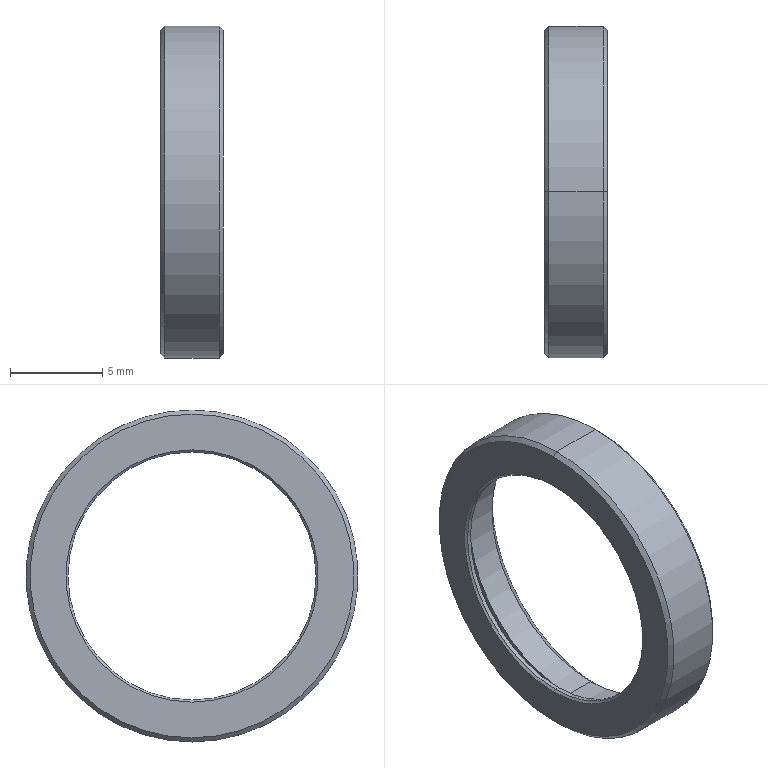Part | SolidWorks | features Revolution 1 | 1 solid | 20 faces | box 3.414 x 18 x 18 mm | volume 239.463 mm3 | cylinder 8 | cone 8 | plane 4 | commonest cylinder face diameters 13.448 x2 15.155 x2 15.951 x2 18 x2
STEP:
#1=CARTESIAN_POINT('',(1545.039,1902.873,9.));
#2=VERTEX_POINT('',#1);
#3=CARTESIAN_POINT('',(1545.039,1902.873,-9.));
#4=VERTEX_POINT('',#3);
#5=CARTESIAN_POINT('',(1545.039,1902.873,0.));
#6=DIRECTION('',(-1.,0.,0.));
#7=DIRECTION('',(0.,0.,1.));
#8=AXIS2_PLACEMENT_3D('',#5,#6,#7);
#9=CIRCLE('',#8,9.);
#10=EDGE_CURVE('',#2,#4,#9,.T.);
#11=ORIENTED_EDGE('',*,*,#10,.T.);
#12=CARTESIAN_POINT('',(1542.08,1902.873,-9.));
#13=VERTEX_POINT('',#12);
#14=CARTESIAN_POINT('',(1539.353,1902.873,-9.));
#15=DIRECTION('',(-1.,0.,0.));
#16=VECTOR('',#15,1000.);
#17=LINE('',#14,#16);
#18=EDGE_CURVE('',#4,#13,#17,.T.);
#19=ORIENTED_EDGE('',*,*,#18,.T.);
#20=CARTESIAN_POINT('',(1542.08,1902.873,9.));
#21=VERTEX_POINT('',#20);
#22=CARTESIAN_POINT('',(1542.08,1902.873,0.));
#23=DIRECTION('',(-1.,0.,0.));
#24=DIRECTION('',(0.,0.,1.));
#25=AXIS2_PLACEMENT_3D('',#22,#23,#24);
#26=CIRCLE('',#25,9.);
#27=EDGE_CURVE('',#21,#13,#26,.T.);
#28=ORIENTED_EDGE('',*,*,#27,.F.);
#29=CARTESIAN_POINT('',(1539.353,1902.873,9.));
#30=DIRECTION('',(-1.,0.,0.));
#31=VECTOR('',#30,1000.);
#32=LINE('',#29,#31);
#33=EDGE_CURVE('',#2,#21,#32,.T.);
#34=ORIENTED_EDGE('',*,*,#33,.F.);
#35=EDGE_LOOP('',(#11,#19,#28,#34));
#36=FACE_OUTER_BOUND('',#35,.T.);
#37=CARTESIAN_POINT('',(1539.353,1902.873,0.));
#38=DIRECTION('',(-1.,0.,0.));
#39=DIRECTION('',(0.,0.,1.));
#40=AXIS2_PLACEMENT_3D('',#37,#38,#39);
#41=CYLINDRICAL_SURFACE('',#40,9.);
#42=ADVANCED_FACE('',(#36),#41,.T.);
#43=CARTESIAN_POINT('',(1541.852,1902.873,8.772));
#44=VERTEX_POINT('',#43);
#45=CARTESIAN_POINT('',(1541.852,1902.873,-8.772));
#46=VERTEX_POINT('',#45);
#47=CARTESIAN_POINT('',(1541.852,1902.873,0.));
#48=DIRECTION('',(-1.,0.,0.));
#49=DIRECTION('',(0.,0.,1.));
#50=AXIS2_PLACEMENT_3D('',#47,#48,#49);
#51=CIRCLE('',#50,8.772);
#52=EDGE_CURVE('',#44,#46,#51,.T.);
#53=ORIENTED_EDGE('',*,*,#52,.F.);
#54=CARTESIAN_POINT('',(1541.852,1902.873,8.772));
#55=DIRECTION('',(0.7071,0.,0.7071));
#56=VECTOR('',#55,1000.);
#57=LINE('',#54,#56);
#58=EDGE_CURVE('',#44,#21,#57,.T.);
#59=ORIENTED_EDGE('',*,*,#58,.T.);
#60=ORIENTED_EDGE('',*,*,#27,.T.);
#61=CARTESIAN_POINT('',(1541.852,1902.873,-8.772));
#62=DIRECTION('',(0.7071,0.,-0.7071));
#63=VECTOR('',#62,1000.);
#64=LINE('',#61,#63);
#65=EDGE_CURVE('',#46,#13,#64,.T.);
#66=ORIENTED_EDGE('',*,*,#65,.F.);
#67=EDGE_LOOP('',(#53,#59,#60,#66));
#68=FACE_OUTER_BOUND('',#67,.T.);
#69=CARTESIAN_POINT('',(1541.852,1902.873,0.));
#70=DIRECTION('',(1.,0.,0.));
#71=DIRECTION('',(0.,0.,-1.));
#72=AXIS2_PLACEMENT_3D('',#69,#70,#71);
#73=CONICAL_SURFACE('',#72,8.772,0.7854);
#74=ADVANCED_FACE('',(#68),#73,.T.);
#75=CARTESIAN_POINT('',(1541.966,1902.873,-6.724));
#76=VERTEX_POINT('',#75);
#77=CARTESIAN_POINT('',(1541.966,1902.873,6.724));
#78=VERTEX_POINT('',#77);
#79=CARTESIAN_POINT('',(1541.966,1902.873,0.));
#80=DIRECTION('',(-1.,0.,0.));
#81=DIRECTION('',(0.,0.,1.));
#82=AXIS2_PLACEMENT_3D('',#79,#80,#81);
#83=CIRCLE('',#82,6.724);
#84=EDGE_CURVE('',#76,#78,#83,.T.);
#85=ORIENTED_EDGE('',*,*,#84,.F.);
#86=CARTESIAN_POINT('',(1541.852,1902.873,-6.838));
#87=VERTEX_POINT('',#86);
#88=CARTESIAN_POINT('',(1541.966,1902.873,-6.724));
#89=DIRECTION('',(-0.7071,0.,-0.7071));
#90=VECTOR('',#89,1000.);
#91=LINE('',#88,#90);
#92=EDGE_CURVE('',#76,#87,#91,.T.);
#93=ORIENTED_EDGE('',*,*,#92,.T.);
#94=CARTESIAN_POINT('',(1541.852,1902.873,6.838));
#95=VERTEX_POINT('',#94);
#96=CARTESIAN_POINT('',(1541.852,1902.873,0.));
#97=DIRECTION('',(-1.,0.,0.));
#98=DIRECTION('',(0.,0.,1.));
#99=AXIS2_PLACEMENT_3D('',#96,#97,#98);
#100=CIRCLE('',#99,6.838);
#101=EDGE_CURVE('',#87,#95,#100,.T.);
#102=ORIENTED_EDGE('',*,*,#101,.T.);
#103=CARTESIAN_POINT('',(1541.966,1902.873,6.724));
#104=DIRECTION('',(-0.7071,0.,0.7071));
#105=VECTOR('',#104,1000.);
#106=LINE('',#103,#105);
#107=EDGE_CURVE('',#78,#95,#106,.T.);
#108=ORIENTED_EDGE('',*,*,#107,.F.);
#109=EDGE_LOOP('',(#85,#93,#102,#108));
#110=FACE_OUTER_BOUND('',#109,.T.);
#111=CARTESIAN_POINT('',(1541.966,1902.873,0.));
#112=DIRECTION('',(-1.,0.,0.));
#113=DIRECTION('',(0.,0.,1.));
#114=AXIS2_PLACEMENT_3D('',#111,#112,#113);
#115=CONICAL_SURFACE('',#114,6.724,0.7854);
#116=ADVANCED_FACE('',(#110),#115,.F.);
#117=CARTESIAN_POINT('',(1542.194,1902.873,-6.724));
#118=VERTEX_POINT('',#117);
#119=CARTESIAN_POINT('',(1542.194,1902.873,6.724));
#120=VERTEX_POINT('',#119);
#121=CARTESIAN_POINT('',(1542.194,1902.873,0.));
#122=DIRECTION('',(-1.,0.,0.));
#123=DIRECTION('',(0.,0.,1.));
#124=AXIS2_PLACEMENT_3D('',#121,#122,#123);
#125=CIRCLE('',#124,6.724);
#126=EDGE_CURVE('',#118,#120,#125,.T.);
#127=ORIENTED_EDGE('',*,*,#126,.F.);
#128=CARTESIAN_POINT('',(1539.353,1902.873,-6.724));
#129=DIRECTION('',(-1.,0.,0.));
#130=VECTOR('',#129,1000.);
#131=LINE('',#128,#130);
#132=EDGE_CURVE('',#118,#76,#131,.T.);
#133=ORIENTED_EDGE('',*,*,#132,.T.);
#134=ORIENTED_EDGE('',*,*,#84,.T.);
#135=CARTESIAN_POINT('',(1539.353,1902.873,6.724));
#136=DIRECTION('',(-1.,0.,0.));
#137=VECTOR('',#136,1000.);
#138=LINE('',#135,#137);
#139=EDGE_CURVE('',#120,#78,#138,.T.);
#140=ORIENTED_EDGE('',*,*,#139,.F.);
#141=EDGE_LOOP('',(#127,#133,#134,#140));
#142=FACE_OUTER_BOUND('',#141,.T.);
#143=CARTESIAN_POINT('',(1539.353,1902.873,0.));
#144=DIRECTION('',(-1.,0.,0.));
#145=DIRECTION('',(0.,0.,1.));
#146=AXIS2_PLACEMENT_3D('',#143,#144,#145);
#147=CYLINDRICAL_SURFACE('',#146,6.724);
#148=ADVANCED_FACE('',(#142),#147,.F.);
#149=CARTESIAN_POINT('',(1542.99,1902.873,-7.976));
#150=VERTEX_POINT('',#149);
#151=CARTESIAN_POINT('',(1542.99,1902.873,7.976));
#152=VERTEX_POINT('',#151);
#153=CARTESIAN_POINT('',(1542.99,1902.873,0.));
#154=DIRECTION('',(-1.,0.,0.));
#155=DIRECTION('',(0.,0.,1.));
#156=AXIS2_PLACEMENT_3D('',#153,#154,#155);
#157=CIRCLE('',#156,7.976);
#158=EDGE_CURVE('',#150,#152,#157,.T.);
#159=ORIENTED_EDGE('',*,*,#158,.F.);
#160=CARTESIAN_POINT('',(1542.194,1902.873,-7.976));
#161=VERTEX_POINT('',#160);
#162=CARTESIAN_POINT('',(1539.353,1902.873,-7.976));
#163=DIRECTION('',(-1.,0.,0.));
#164=VECTOR('',#163,1000.);
#165=LINE('',#162,#164);
#166=EDGE_CURVE('',#150,#161,#165,.T.);
#167=ORIENTED_EDGE('',*,*,#166,.T.);
#168=CARTESIAN_POINT('',(1542.194,1902.873,7.976));
#169=VERTEX_POINT('',#168);
#170=CARTESIAN_POINT('',(1542.194,1902.873,0.));
#171=DIRECTION('',(-1.,0.,0.));
#172=DIRECTION('',(0.,0.,1.));
#173=AXIS2_PLACEMENT_3D('',#170,#171,#172);
#174=CIRCLE('',#173,7.976);
#175=EDGE_CURVE('',#161,#169,#174,.T.);
#176=ORIENTED_EDGE('',*,*,#175,.T.);
#177=CARTESIAN_POINT('',(1539.353,1902.873,7.976));
#178=DIRECTION('',(-1.,0.,0.));
#179=VECTOR('',#178,1000.);
#180=LINE('',#177,#179);
#181=EDGE_CURVE('',#152,#169,#180,.T.);
#182=ORIENTED_EDGE('',*,*,#181,.F.);
#183=EDGE_LOOP('',(#159,#167,#176,#182));
#184=FACE_OUTER_BOUND('',#183,.T.);
#185=CARTESIAN_POINT('',(1539.353,1902.873,0.));
#186=DIRECTION('',(-1.,0.,0.));
#187=DIRECTION('',(0.,0.,1.));
#188=AXIS2_PLACEMENT_3D('',#185,#186,#187);
#189=CYLINDRICAL_SURFACE('',#188,7.976);
#190=ADVANCED_FACE('',(#184),#189,.F.);
#191=CARTESIAN_POINT('',(1544.697,1902.873,-7.577));
#192=VERTEX_POINT('',#191);
#193=CARTESIAN_POINT('',(1544.697,1902.873,7.577));
#194=VERTEX_POINT('',#193);
#195=CARTESIAN_POINT('',(1544.697,1902.873,0.));
#196=DIRECTION('',(-1.,0.,0.));
#197=DIRECTION('',(0.,0.,1.));
#198=AXIS2_PLACEMENT_3D('',#195,#196,#197);
#199=CIRCLE('',#198,7.577);
#200=EDGE_CURVE('',#192,#194,#199,.T.);
#201=ORIENTED_EDGE('',*,*,#200,.F.);
#202=CARTESIAN_POINT('',(1542.99,1902.873,-7.577));
#203=VERTEX_POINT('',#202);
#204=CARTESIAN_POINT('',(1539.353,1902.873,-7.577));
#205=DIRECTION('',(-1.,0.,0.));
#206=VECTOR('',#205,1000.);
#207=LINE('',#204,#206);
#208=EDGE_CURVE('',#192,#203,#207,.T.);
#209=ORIENTED_EDGE('',*,*,#208,.T.);
#210=CARTESIAN_POINT('',(1542.99,1902.873,7.577));
#211=VERTEX_POINT('',#210);
#212=CARTESIAN_POINT('',(1542.99,1902.873,0.));
#213=DIRECTION('',(-1.,0.,0.));
#214=DIRECTION('',(0.,0.,1.));
#215=AXIS2_PLACEMENT_3D('',#212,#213,#214);
#216=CIRCLE('',#215,7.577);
#217=EDGE_CURVE('',#203,#211,#216,.T.);
#218=ORIENTED_EDGE('',*,*,#217,.T.);
#219=CARTESIAN_POINT('',(1539.353,1902.873,7.577));
#220=DIRECTION('',(-1.,0.,0.));
#221=VECTOR('',#220,1000.);
#222=LINE('',#219,#221);
#223=EDGE_CURVE('',#194,#211,#222,.T.);
#224=ORIENTED_EDGE('',*,*,#223,.F.);
#225=EDGE_LOOP('',(#201,#209,#218,#224));
#226=FACE_OUTER_BOUND('',#225,.T.);
#227=CARTESIAN_POINT('',(1539.353,1902.873,0.));
#228=DIRECTION('',(-1.,0.,0.));
#229=DIRECTION('',(0.,0.,1.));
#230=AXIS2_PLACEMENT_3D('',#227,#228,#229);
#231=CYLINDRICAL_SURFACE('',#230,7.577);
#232=ADVANCED_FACE('',(#226),#231,.F.);
#233=ORIENTED_EDGE('',*,*,#200,.T.);
#234=CARTESIAN_POINT('',(1545.266,1902.873,8.146));
#235=VERTEX_POINT('',#234);
#236=CARTESIAN_POINT('',(1545.266,1902.873,8.146));
#237=DIRECTION('',(0.7071,0.,0.7071));
#238=VECTOR('',#237,1000.);
#239=LINE('',#236,#238);
#240=EDGE_CURVE('',#194,#235,#239,.T.);
#241=ORIENTED_EDGE('',*,*,#240,.T.);
#242=CARTESIAN_POINT('',(1545.266,1902.873,-8.146));
#243=VERTEX_POINT('',#242);
#244=CARTESIAN_POINT('',(1545.266,1902.873,0.));
#245=DIRECTION('',(-1.,0.,0.));
#246=DIRECTION('',(0.,0.,1.));
#247=AXIS2_PLACEMENT_3D('',#244,#245,#246);
#248=CIRCLE('',#247,8.146);
#249=EDGE_CURVE('',#243,#235,#248,.T.);
#250=ORIENTED_EDGE('',*,*,#249,.F.);
#251=CARTESIAN_POINT('',(1545.266,1902.873,-8.146));
#252=DIRECTION('',(0.7071,0.,-0.7071));
#253=VECTOR('',#252,1000.);
#254=LINE('',#251,#253);
#255=EDGE_CURVE('',#192,#243,#254,.T.);
#256=ORIENTED_EDGE('',*,*,#255,.F.);
#257=EDGE_LOOP('',(#233,#241,#250,#256));
#258=FACE_OUTER_BOUND('',#257,.T.);
#259=CARTESIAN_POINT('',(1545.266,1902.873,0.));
#260=DIRECTION('',(1.,0.,0.));
#261=DIRECTION('',(0.,0.,-1.));
#262=AXIS2_PLACEMENT_3D('',#259,#260,#261);
#263=CONICAL_SURFACE('',#262,8.146,0.7854);
#264=ADVANCED_FACE('',(#258),#263,.F.);
#265=CARTESIAN_POINT('',(1545.266,1902.873,8.772));
#266=VERTEX_POINT('',#265);
#267=CARTESIAN_POINT('',(1545.266,1902.873,-8.772));
#268=VERTEX_POINT('',#267);
#269=CARTESIAN_POINT('',(1545.266,1902.873,0.));
#270=DIRECTION('',(-1.,0.,0.));
#271=DIRECTION('',(0.,0.,1.));
#272=AXIS2_PLACEMENT_3D('',#269,#270,#271);
#273=CIRCLE('',#272,8.772);
#274=EDGE_CURVE('',#266,#268,#273,.T.);
#275=ORIENTED_EDGE('',*,*,#274,.T.);
#276=CARTESIAN_POINT('',(1545.266,1902.873,-8.772));
#277=DIRECTION('',(-0.7071,0.,-0.7071));
#278=VECTOR('',#277,1000.);
#279=LINE('',#276,#278);
#280=EDGE_CURVE('',#268,#4,#279,.T.);
#281=ORIENTED_EDGE('',*,*,#280,.T.);
#282=ORIENTED_EDGE('',*,*,#10,.F.);
#283=CARTESIAN_POINT('',(1545.266,1902.873,8.772));
#284=DIRECTION('',(-0.7071,0.,0.7071));
#285=VECTOR('',#284,1000.);
#286=LINE('',#283,#285);
#287=EDGE_CURVE('',#266,#2,#286,.T.);
#288=ORIENTED_EDGE('',*,*,#287,.F.);
#289=EDGE_LOOP('',(#275,#281,#282,#288));
#290=FACE_OUTER_BOUND('',#289,.T.);
#291=CARTESIAN_POINT('',(1545.266,1902.873,0.));
#292=DIRECTION('',(-1.,0.,0.));
#293=DIRECTION('',(0.,0.,1.));
#294=AXIS2_PLACEMENT_3D('',#291,#292,#293);
#295=CONICAL_SURFACE('',#294,8.772,0.7854);
#296=ADVANCED_FACE('',(#290),#295,.T.);
#297=ORIENTED_EDGE('',*,*,#280,.F.);
#298=CARTESIAN_POINT('',(1545.266,1902.873,0.));
#299=DIRECTION('',(-1.,0.,0.));
#300=DIRECTION('',(0.,0.,1.));
#301=AXIS2_PLACEMENT_3D('',#298,#299,#300);
#302=CIRCLE('',#301,8.772);
#303=EDGE_CURVE('',#268,#266,#302,.T.);
#304=ORIENTED_EDGE('',*,*,#303,.T.);
#305=ORIENTED_EDGE('',*,*,#287,.T.);
#306=CARTESIAN_POINT('',(1545.039,1902.873,0.));
#307=DIRECTION('',(-1.,0.,0.));
#308=DIRECTION('',(0.,0.,1.));
#309=AXIS2_PLACEMENT_3D('',#306,#307,#308);
#310=CIRCLE('',#309,9.);
#311=EDGE_CURVE('',#4,#2,#310,.T.);
#312=ORIENTED_EDGE('',*,*,#311,.F.);
#313=EDGE_LOOP('',(#297,#304,#305,#312));
#314=FACE_OUTER_BOUND('',#313,.T.);
#315=CARTESIAN_POINT('',(1545.266,1902.873,0.));
#316=DIRECTION('',(-1.,0.,0.));
#317=DIRECTION('',(0.,0.,1.));
#318=AXIS2_PLACEMENT_3D('',#315,#316,#317);
#319=CONICAL_SURFACE('',#318,8.772,0.7854);
#320=ADVANCED_FACE('',(#314),#319,.T.);
#321=ORIENTED_EDGE('',*,*,#274,.F.);
#322=ORIENTED_EDGE('',*,*,#303,.F.);
#323=EDGE_LOOP('',(#321,#322));
#324=FACE_OUTER_BOUND('',#323,.T.);
#325=ORIENTED_EDGE('',*,*,#249,.T.);
#326=CARTESIAN_POINT('',(1545.266,1902.873,0.));
#327=DIRECTION('',(-1.,0.,0.));
#328=DIRECTION('',(0.,0.,1.));
#329=AXIS2_PLACEMENT_3D('',#326,#327,#328);
#330=CIRCLE('',#329,8.146);
#331=EDGE_CURVE('',#235,#243,#330,.T.);
#332=ORIENTED_EDGE('',*,*,#331,.T.);
#333=EDGE_LOOP('',(#325,#332));
#334=FACE_BOUND('',#333,.T.);
#335=CARTESIAN_POINT('',(1545.266,-0.000000002,0.));
#336=DIRECTION('',(-1.,0.,0.));
#337=DIRECTION('',(0.,0.,1.));
#338=AXIS2_PLACEMENT_3D('',#335,#336,#337);
#339=PLANE('',#338);
#340=ADVANCED_FACE('',(#324,#334),#339,.F.);
#341=ORIENTED_EDGE('',*,*,#240,.F.);
#342=CARTESIAN_POINT('',(1544.697,1902.873,0.));
#343=DIRECTION('',(-1.,0.,0.));
#344=DIRECTION('',(0.,0.,1.));
#345=AXIS2_PLACEMENT_3D('',#342,#343,#344);
#346=CIRCLE('',#345,7.577);
#347=EDGE_CURVE('',#194,#192,#346,.T.);
#348=ORIENTED_EDGE('',*,*,#347,.T.);
#349=ORIENTED_EDGE('',*,*,#255,.T.);
#350=ORIENTED_EDGE('',*,*,#331,.F.);
#351=EDGE_LOOP('',(#341,#348,#349,#350));
#352=FACE_OUTER_BOUND('',#351,.T.);
#353=CARTESIAN_POINT('',(1545.266,1902.873,0.));
#354=DIRECTION('',(1.,0.,0.));
#355=DIRECTION('',(0.,0.,-1.));
#356=AXIS2_PLACEMENT_3D('',#353,#354,#355);
#357=CONICAL_SURFACE('',#356,8.146,0.7854);
#358=ADVANCED_FACE('',(#352),#357,.F.);
#359=ORIENTED_EDGE('',*,*,#208,.F.);
#360=ORIENTED_EDGE('',*,*,#347,.F.);
#361=ORIENTED_EDGE('',*,*,#223,.T.);
#362=CARTESIAN_POINT('',(1542.99,1902.873,0.));
#363=DIRECTION('',(-1.,0.,0.));
#364=DIRECTION('',(0.,0.,1.));
#365=AXIS2_PLACEMENT_3D('',#362,#363,#364);
#366=CIRCLE('',#365,7.577);
#367=EDGE_CURVE('',#211,#203,#366,.T.);
#368=ORIENTED_EDGE('',*,*,#367,.T.);
#369=EDGE_LOOP('',(#359,#360,#361,#368));
#370=FACE_OUTER_BOUND('',#369,.T.);
#371=CARTESIAN_POINT('',(1539.353,1902.873,0.));
#372=DIRECTION('',(-1.,0.,0.));
#373=DIRECTION('',(0.,0.,1.));
#374=AXIS2_PLACEMENT_3D('',#371,#372,#373);
#375=CYLINDRICAL_SURFACE('',#374,7.577);
#376=ADVANCED_FACE('',(#370),#375,.F.);
#377=CARTESIAN_POINT('',(1542.99,1902.873,0.));
#378=DIRECTION('',(-1.,0.,0.));
#379=DIRECTION('',(0.,0.,1.));
#380=AXIS2_PLACEMENT_3D('',#377,#378,#379);
#381=CIRCLE('',#380,7.976);
#382=EDGE_CURVE('',#152,#150,#381,.T.);
#383=ORIENTED_EDGE('',*,*,#382,.T.);
#384=ORIENTED_EDGE('',*,*,#158,.T.);
#385=EDGE_LOOP('',(#383,#384));
#386=FACE_OUTER_BOUND('',#385,.T.);
#387=ORIENTED_EDGE('',*,*,#367,.F.);
#388=ORIENTED_EDGE('',*,*,#217,.F.);
#389=EDGE_LOOP('',(#387,#388));
#390=FACE_BOUND('',#389,.T.);
#391=CARTESIAN_POINT('',(1542.99,0.,0.));
#392=DIRECTION('',(-1.,0.,0.));
#393=DIRECTION('',(0.,0.,1.));
#394=AXIS2_PLACEMENT_3D('',#391,#392,#393);
#395=PLANE('',#394);
#396=ADVANCED_FACE('',(#386,#390),#395,.T.);
#397=ORIENTED_EDGE('',*,*,#166,.F.);
#398=ORIENTED_EDGE('',*,*,#382,.F.);
#399=ORIENTED_EDGE('',*,*,#181,.T.);
#400=CARTESIAN_POINT('',(1542.194,1902.873,0.));
#401=DIRECTION('',(-1.,0.,0.));
#402=DIRECTION('',(0.,0.,1.));
#403=AXIS2_PLACEMENT_3D('',#400,#401,#402);
#404=CIRCLE('',#403,7.976);
#405=EDGE_CURVE('',#169,#161,#404,.T.);
#406=ORIENTED_EDGE('',*,*,#405,.T.);
#407=EDGE_LOOP('',(#397,#398,#399,#406));
#408=FACE_OUTER_BOUND('',#407,.T.);
#409=CARTESIAN_POINT('',(1539.353,1902.873,0.));
#410=DIRECTION('',(-1.,0.,0.));
#411=DIRECTION('',(0.,0.,1.));
#412=AXIS2_PLACEMENT_3D('',#409,#410,#411);
#413=CYLINDRICAL_SURFACE('',#412,7.976);
#414=ADVANCED_FACE('',(#408),#413,.F.);
#415=ORIENTED_EDGE('',*,*,#405,.F.);
#416=ORIENTED_EDGE('',*,*,#175,.F.);
#417=EDGE_LOOP('',(#415,#416));
#418=FACE_OUTER_BOUND('',#417,.T.);
#419=CARTESIAN_POINT('',(1542.194,1902.873,0.));
#420=DIRECTION('',(-1.,0.,0.));
#421=DIRECTION('',(0.,0.,1.));
#422=AXIS2_PLACEMENT_3D('',#419,#420,#421);
#423=CIRCLE('',#422,6.724);
#424=EDGE_CURVE('',#120,#118,#423,.T.);
#425=ORIENTED_EDGE('',*,*,#424,.T.);
#426=ORIENTED_EDGE('',*,*,#126,.T.);
#427=EDGE_LOOP('',(#425,#426));
#428=FACE_BOUND('',#427,.T.);
#429=CARTESIAN_POINT('',(1542.194,0.,0.));
#430=DIRECTION('',(-1.,0.,0.));
#431=DIRECTION('',(0.,0.,1.));
#432=AXIS2_PLACEMENT_3D('',#429,#430,#431);
#433=PLANE('',#432);
#434=ADVANCED_FACE('',(#418,#428),#433,.F.);
#435=ORIENTED_EDGE('',*,*,#132,.F.);
#436=ORIENTED_EDGE('',*,*,#424,.F.);
#437=ORIENTED_EDGE('',*,*,#139,.T.);
#438=CARTESIAN_POINT('',(1541.966,1902.873,0.));
#439=DIRECTION('',(-1.,0.,0.));
#440=DIRECTION('',(0.,0.,1.));
#441=AXIS2_PLACEMENT_3D('',#438,#439,#440);
#442=CIRCLE('',#441,6.724);
#443=EDGE_CURVE('',#78,#76,#442,.T.);
#444=ORIENTED_EDGE('',*,*,#443,.T.);
#445=EDGE_LOOP('',(#435,#436,#437,#444));
#446=FACE_OUTER_BOUND('',#445,.T.);
#447=CARTESIAN_POINT('',(1539.353,1902.873,0.));
#448=DIRECTION('',(-1.,0.,0.));
#449=DIRECTION('',(0.,0.,1.));
#450=AXIS2_PLACEMENT_3D('',#447,#448,#449);
#451=CYLINDRICAL_SURFACE('',#450,6.724);
#452=ADVANCED_FACE('',(#446),#451,.F.);
#453=ORIENTED_EDGE('',*,*,#92,.F.);
#454=ORIENTED_EDGE('',*,*,#443,.F.);
#455=ORIENTED_EDGE('',*,*,#107,.T.);
#456=CARTESIAN_POINT('',(1541.852,1902.873,0.));
#457=DIRECTION('',(-1.,0.,0.));
#458=DIRECTION('',(0.,0.,1.));
#459=AXIS2_PLACEMENT_3D('',#456,#457,#458);
#460=CIRCLE('',#459,6.838);
#461=EDGE_CURVE('',#95,#87,#460,.T.);
#462=ORIENTED_EDGE('',*,*,#461,.T.);
#463=EDGE_LOOP('',(#453,#454,#455,#462));
#464=FACE_OUTER_BOUND('',#463,.T.);
#465=CARTESIAN_POINT('',(1541.966,1902.873,0.));
#466=DIRECTION('',(-1.,0.,0.));
#467=DIRECTION('',(0.,0.,1.));
#468=AXIS2_PLACEMENT_3D('',#465,#466,#467);
#469=CONICAL_SURFACE('',#468,6.724,0.7854);
#470=ADVANCED_FACE('',(#464),#469,.F.);
#471=CARTESIAN_POINT('',(1541.852,1902.873,0.));
#472=DIRECTION('',(-1.,0.,0.));
#473=DIRECTION('',(0.,0.,1.));
#474=AXIS2_PLACEMENT_3D('',#471,#472,#473);
#475=CIRCLE('',#474,8.772);
#476=EDGE_CURVE('',#46,#44,#475,.T.);
#477=ORIENTED_EDGE('',*,*,#476,.T.);
#478=ORIENTED_EDGE('',*,*,#52,.T.);
#479=EDGE_LOOP('',(#477,#478));
#480=FACE_OUTER_BOUND('',#479,.T.);
#481=ORIENTED_EDGE('',*,*,#461,.F.);
#482=ORIENTED_EDGE('',*,*,#101,.F.);
#483=EDGE_LOOP('',(#481,#482));
#484=FACE_BOUND('',#483,.T.);
#485=CARTESIAN_POINT('',(1541.852,0.,0.));
#486=DIRECTION('',(-1.,0.,0.));
#487=DIRECTION('',(0.,0.,1.));
#488=AXIS2_PLACEMENT_3D('',#485,#486,#487);
#489=PLANE('',#488);
#490=ADVANCED_FACE('',(#480,#484),#489,.T.);
#491=ORIENTED_EDGE('',*,*,#58,.F.);
#492=ORIENTED_EDGE('',*,*,#476,.F.);
#493=ORIENTED_EDGE('',*,*,#65,.T.);
#494=CARTESIAN_POINT('',(1542.08,1902.873,0.));
#495=DIRECTION('',(-1.,0.,0.));
#496=DIRECTION('',(0.,0.,1.));
#497=AXIS2_PLACEMENT_3D('',#494,#495,#496);
#498=CIRCLE('',#497,9.);
#499=EDGE_CURVE('',#13,#21,#498,.T.);
#500=ORIENTED_EDGE('',*,*,#499,.T.);
#501=EDGE_LOOP('',(#491,#492,#493,#500));
#502=FACE_OUTER_BOUND('',#501,.T.);
#503=CARTESIAN_POINT('',(1541.852,1902.873,0.));
#504=DIRECTION('',(1.,0.,0.));
#505=DIRECTION('',(0.,0.,-1.));
#506=AXIS2_PLACEMENT_3D('',#503,#504,#505);
#507=CONICAL_SURFACE('',#506,8.772,0.7854);
#508=ADVANCED_FACE('',(#502),#507,.T.);
#509=ORIENTED_EDGE('',*,*,#18,.F.);
#510=ORIENTED_EDGE('',*,*,#311,.T.);
#511=ORIENTED_EDGE('',*,*,#33,.T.);
#512=ORIENTED_EDGE('',*,*,#499,.F.);
#513=EDGE_LOOP('',(#509,#510,#511,#512));
#514=FACE_OUTER_BOUND('',#513,.T.);
#515=CARTESIAN_POINT('',(1539.353,1902.873,0.));
#516=DIRECTION('',(-1.,0.,0.));
#517=DIRECTION('',(0.,0.,1.));
#518=AXIS2_PLACEMENT_3D('',#515,#516,#517);
#519=CYLINDRICAL_SURFACE('',#518,9.);
#520=ADVANCED_FACE('',(#514),#519,.T.);
#521=CLOSED_SHELL('',(#42,#74,#116,#148,#190,#232,#264,#296,#320,#340,#358,#376,#396,#414,#434,#452,#470,#490,#508,#520));
#522=MANIFOLD_SOLID_BREP('',#521);
#523=CARTESIAN_POINT('',(0.,0.,0.));
#524=DIRECTION('',(0.,0.,1.));
#525=DIRECTION('',(1.,0.,0.));
#526=AXIS2_PLACEMENT_3D('',#523,#524,#525);
#527=(LENGTH_UNIT()NAMED_UNIT(*)SI_UNIT(.MILLI.,.METRE.));
#528=UNCERTAINTY_MEASURE_WITH_UNIT(LENGTH_MEASURE(0.00001),#527,'','');
#529=(NAMED_UNIT(*)PLANE_ANGLE_UNIT()SI_UNIT($,.RADIAN.));
#530=(NAMED_UNIT(*)SI_UNIT($,.STERADIAN.)SOLID_ANGLE_UNIT());
#531=(GEOMETRIC_REPRESENTATION_CONTEXT(3)GLOBAL_UNCERTAINTY_ASSIGNED_CONTEXT((#528))GLOBAL_UNIT_ASSIGNED_CONTEXT((#527,#529,#530))REPRESENTATION_CONTEXT('',''));
#532=ADVANCED_BREP_SHAPE_REPRESENTATION('',(#522,#526),#531);